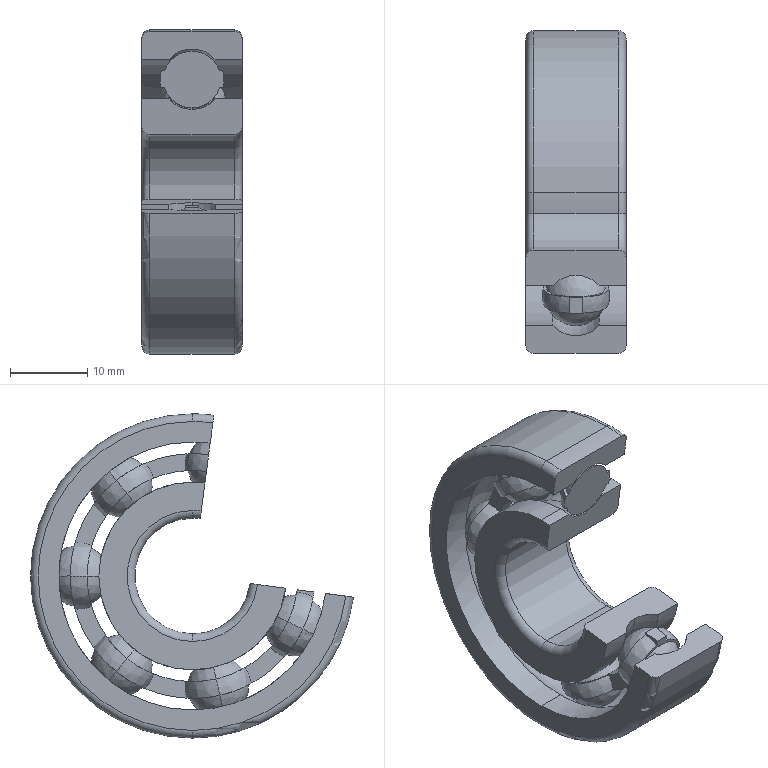Part | STEP file | Bearing 6302 | 1 solid | 125 faces | box 13 x 41.82 x 42 mm | volume 7834 mm3 | sphere 44 | torus 33 | cylinder 26 | plane 22 | commonest cylinder face diameters 24.3 x6 34.7 x6 27.317 x4 31.683 x4 15 x3 42 x3